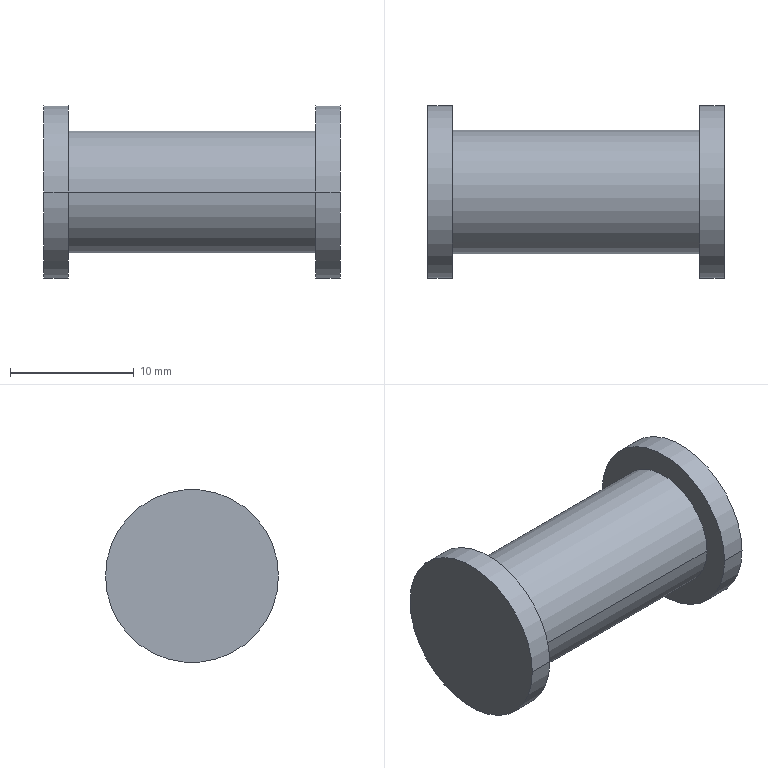Part | SolidWorks | 1 solid | 10 faces | box 24 x 14 x 14 mm | volume 2187 mm3 | cylinder 6 | plane 4 | commonest cylinder face diameters 14 x4 10 x2
STEP:
#1=CARTESIAN_POINT('',(-10.,-7.,0.));
#2=VERTEX_POINT('',#1);
#3=CARTESIAN_POINT('',(-10.,7.,0.));
#4=VERTEX_POINT('',#3);
#5=CARTESIAN_POINT('',(-10.,0.,0.));
#6=DIRECTION('',(-1.,0.,0.));
#7=DIRECTION('',(0.,-1.,0.));
#8=AXIS2_PLACEMENT_3D('',#5,#6,#7);
#9=CIRCLE('',#8,7.);
#10=EDGE_CURVE('',#2,#4,#9,.T.);
#11=ORIENTED_EDGE('',*,*,#10,.T.);
#12=CARTESIAN_POINT('',(-12.,7.,0.));
#13=VERTEX_POINT('',#12);
#14=CARTESIAN_POINT('',(0.,7.,0.));
#15=DIRECTION('',(-1.,0.,0.));
#16=VECTOR('',#15,1000.);
#17=LINE('',#14,#16);
#18=EDGE_CURVE('',#4,#13,#17,.T.);
#19=ORIENTED_EDGE('',*,*,#18,.T.);
#20=CARTESIAN_POINT('',(-12.,-7.,0.));
#21=VERTEX_POINT('',#20);
#22=CARTESIAN_POINT('',(-12.,0.,0.));
#23=DIRECTION('',(-1.,0.,0.));
#24=DIRECTION('',(0.,-1.,0.));
#25=AXIS2_PLACEMENT_3D('',#22,#23,#24);
#26=CIRCLE('',#25,7.);
#27=EDGE_CURVE('',#21,#13,#26,.T.);
#28=ORIENTED_EDGE('',*,*,#27,.F.);
#29=CARTESIAN_POINT('',(0.,-7.,0.));
#30=DIRECTION('',(-1.,0.,0.));
#31=VECTOR('',#30,1000.);
#32=LINE('',#29,#31);
#33=EDGE_CURVE('',#2,#21,#32,.T.);
#34=ORIENTED_EDGE('',*,*,#33,.F.);
#35=EDGE_LOOP('',(#11,#19,#28,#34));
#36=FACE_OUTER_BOUND('',#35,.T.);
#37=CARTESIAN_POINT('',(0.,0.,0.));
#38=DIRECTION('',(-1.,0.,0.));
#39=DIRECTION('',(0.,-1.,0.));
#40=AXIS2_PLACEMENT_3D('',#37,#38,#39);
#41=CYLINDRICAL_SURFACE('',#40,7.);
#42=ADVANCED_FACE('',(#36),#41,.T.);
#43=CARTESIAN_POINT('',(12.,-7.,0.));
#44=VERTEX_POINT('',#43);
#45=CARTESIAN_POINT('',(12.,7.,0.));
#46=VERTEX_POINT('',#45);
#47=CARTESIAN_POINT('',(12.,0.,0.));
#48=DIRECTION('',(-1.,0.,0.));
#49=DIRECTION('',(0.,-1.,0.));
#50=AXIS2_PLACEMENT_3D('',#47,#48,#49);
#51=CIRCLE('',#50,7.);
#52=EDGE_CURVE('',#44,#46,#51,.T.);
#53=ORIENTED_EDGE('',*,*,#52,.T.);
#54=CARTESIAN_POINT('',(10.,7.,0.));
#55=VERTEX_POINT('',#54);
#56=CARTESIAN_POINT('',(0.,7.,0.));
#57=DIRECTION('',(-1.,0.,0.));
#58=VECTOR('',#57,1000.);
#59=LINE('',#56,#58);
#60=EDGE_CURVE('',#46,#55,#59,.T.);
#61=ORIENTED_EDGE('',*,*,#60,.T.);
#62=CARTESIAN_POINT('',(10.,-7.,0.));
#63=VERTEX_POINT('',#62);
#64=CARTESIAN_POINT('',(10.,0.,0.));
#65=DIRECTION('',(-1.,0.,0.));
#66=DIRECTION('',(0.,-1.,0.));
#67=AXIS2_PLACEMENT_3D('',#64,#65,#66);
#68=CIRCLE('',#67,7.);
#69=EDGE_CURVE('',#63,#55,#68,.T.);
#70=ORIENTED_EDGE('',*,*,#69,.F.);
#71=CARTESIAN_POINT('',(0.,-7.,0.));
#72=DIRECTION('',(-1.,0.,0.));
#73=VECTOR('',#72,1000.);
#74=LINE('',#71,#73);
#75=EDGE_CURVE('',#44,#63,#74,.T.);
#76=ORIENTED_EDGE('',*,*,#75,.F.);
#77=EDGE_LOOP('',(#53,#61,#70,#76));
#78=FACE_OUTER_BOUND('',#77,.T.);
#79=CARTESIAN_POINT('',(0.,0.,0.));
#80=DIRECTION('',(-1.,0.,0.));
#81=DIRECTION('',(0.,-1.,0.));
#82=AXIS2_PLACEMENT_3D('',#79,#80,#81);
#83=CYLINDRICAL_SURFACE('',#82,7.);
#84=ADVANCED_FACE('',(#78),#83,.T.);
#85=CARTESIAN_POINT('',(10.,-5.,0.));
#86=VERTEX_POINT('',#85);
#87=CARTESIAN_POINT('',(10.,5.,0.));
#88=VERTEX_POINT('',#87);
#89=CARTESIAN_POINT('',(10.,0.,0.));
#90=DIRECTION('',(-1.,0.,0.));
#91=DIRECTION('',(0.,-1.,0.));
#92=AXIS2_PLACEMENT_3D('',#89,#90,#91);
#93=CIRCLE('',#92,5.);
#94=EDGE_CURVE('',#86,#88,#93,.T.);
#95=ORIENTED_EDGE('',*,*,#94,.T.);
#96=CARTESIAN_POINT('',(-10.,5.,0.));
#97=VERTEX_POINT('',#96);
#98=CARTESIAN_POINT('',(0.,5.,0.));
#99=DIRECTION('',(-1.,0.,0.));
#100=VECTOR('',#99,1000.);
#101=LINE('',#98,#100);
#102=EDGE_CURVE('',#88,#97,#101,.T.);
#103=ORIENTED_EDGE('',*,*,#102,.T.);
#104=CARTESIAN_POINT('',(-10.,-5.,0.));
#105=VERTEX_POINT('',#104);
#106=CARTESIAN_POINT('',(-10.,0.,0.));
#107=DIRECTION('',(-1.,0.,0.));
#108=DIRECTION('',(0.,-1.,0.));
#109=AXIS2_PLACEMENT_3D('',#106,#107,#108);
#110=CIRCLE('',#109,5.);
#111=EDGE_CURVE('',#105,#97,#110,.T.);
#112=ORIENTED_EDGE('',*,*,#111,.F.);
#113=CARTESIAN_POINT('',(0.,-5.,0.));
#114=DIRECTION('',(-1.,0.,0.));
#115=VECTOR('',#114,1000.);
#116=LINE('',#113,#115);
#117=EDGE_CURVE('',#86,#105,#116,.T.);
#118=ORIENTED_EDGE('',*,*,#117,.F.);
#119=EDGE_LOOP('',(#95,#103,#112,#118));
#120=FACE_OUTER_BOUND('',#119,.T.);
#121=CARTESIAN_POINT('',(0.,0.,0.));
#122=DIRECTION('',(-1.,0.,0.));
#123=DIRECTION('',(0.,-1.,0.));
#124=AXIS2_PLACEMENT_3D('',#121,#122,#123);
#125=CYLINDRICAL_SURFACE('',#124,5.);
#126=ADVANCED_FACE('',(#120),#125,.T.);
#127=ORIENTED_EDGE('',*,*,#10,.F.);
#128=CARTESIAN_POINT('',(-10.,0.,0.));
#129=DIRECTION('',(-1.,0.,0.));
#130=DIRECTION('',(0.,-1.,0.));
#131=AXIS2_PLACEMENT_3D('',#128,#129,#130);
#132=CIRCLE('',#131,7.);
#133=EDGE_CURVE('',#4,#2,#132,.T.);
#134=ORIENTED_EDGE('',*,*,#133,.F.);
#135=EDGE_LOOP('',(#127,#134));
#136=FACE_OUTER_BOUND('',#135,.T.);
#137=ORIENTED_EDGE('',*,*,#111,.T.);
#138=CARTESIAN_POINT('',(-10.,0.,0.));
#139=DIRECTION('',(-1.,0.,0.));
#140=DIRECTION('',(0.,-1.,0.));
#141=AXIS2_PLACEMENT_3D('',#138,#139,#140);
#142=CIRCLE('',#141,5.);
#143=EDGE_CURVE('',#97,#105,#142,.T.);
#144=ORIENTED_EDGE('',*,*,#143,.T.);
#145=EDGE_LOOP('',(#137,#144));
#146=FACE_BOUND('',#145,.T.);
#147=CARTESIAN_POINT('',(-10.,5.,0.));
#148=DIRECTION('',(-1.,0.,0.));
#149=DIRECTION('',(0.,-1.,0.));
#150=AXIS2_PLACEMENT_3D('',#147,#148,#149);
#151=PLANE('',#150);
#152=ADVANCED_FACE('',(#136,#146),#151,.F.);
#153=ORIENTED_EDGE('',*,*,#102,.F.);
#154=CARTESIAN_POINT('',(10.,0.,0.));
#155=DIRECTION('',(-1.,0.,0.));
#156=DIRECTION('',(0.,-1.,0.));
#157=AXIS2_PLACEMENT_3D('',#154,#155,#156);
#158=CIRCLE('',#157,5.);
#159=EDGE_CURVE('',#88,#86,#158,.T.);
#160=ORIENTED_EDGE('',*,*,#159,.T.);
#161=ORIENTED_EDGE('',*,*,#117,.T.);
#162=ORIENTED_EDGE('',*,*,#143,.F.);
#163=EDGE_LOOP('',(#153,#160,#161,#162));
#164=FACE_OUTER_BOUND('',#163,.T.);
#165=CARTESIAN_POINT('',(0.,0.,0.));
#166=DIRECTION('',(-1.,0.,0.));
#167=DIRECTION('',(0.,-1.,0.));
#168=AXIS2_PLACEMENT_3D('',#165,#166,#167);
#169=CYLINDRICAL_SURFACE('',#168,5.);
#170=ADVANCED_FACE('',(#164),#169,.T.);
#171=ORIENTED_EDGE('',*,*,#94,.F.);
#172=ORIENTED_EDGE('',*,*,#159,.F.);
#173=EDGE_LOOP('',(#171,#172));
#174=FACE_BOUND('',#173,.T.);
#175=ORIENTED_EDGE('',*,*,#69,.T.);
#176=CARTESIAN_POINT('',(10.,0.,0.));
#177=DIRECTION('',(-1.,0.,0.));
#178=DIRECTION('',(0.,-1.,0.));
#179=AXIS2_PLACEMENT_3D('',#176,#177,#178);
#180=CIRCLE('',#179,7.);
#181=EDGE_CURVE('',#55,#63,#180,.T.);
#182=ORIENTED_EDGE('',*,*,#181,.T.);
#183=EDGE_LOOP('',(#175,#182));
#184=FACE_OUTER_BOUND('',#183,.T.);
#185=CARTESIAN_POINT('',(10.,5.,0.));
#186=DIRECTION('',(1.,0.,0.));
#187=DIRECTION('',(0.,1.,0.));
#188=AXIS2_PLACEMENT_3D('',#185,#186,#187);
#189=PLANE('',#188);
#190=ADVANCED_FACE('',(#174,#184),#189,.F.);
#191=ORIENTED_EDGE('',*,*,#60,.F.);
#192=CARTESIAN_POINT('',(12.,0.,0.));
#193=DIRECTION('',(-1.,0.,0.));
#194=DIRECTION('',(0.,-1.,0.));
#195=AXIS2_PLACEMENT_3D('',#192,#193,#194);
#196=CIRCLE('',#195,7.);
#197=EDGE_CURVE('',#46,#44,#196,.T.);
#198=ORIENTED_EDGE('',*,*,#197,.T.);
#199=ORIENTED_EDGE('',*,*,#75,.T.);
#200=ORIENTED_EDGE('',*,*,#181,.F.);
#201=EDGE_LOOP('',(#191,#198,#199,#200));
#202=FACE_OUTER_BOUND('',#201,.T.);
#203=CARTESIAN_POINT('',(0.,0.,0.));
#204=DIRECTION('',(-1.,0.,0.));
#205=DIRECTION('',(0.,-1.,0.));
#206=AXIS2_PLACEMENT_3D('',#203,#204,#205);
#207=CYLINDRICAL_SURFACE('',#206,7.);
#208=ADVANCED_FACE('',(#202),#207,.T.);
#209=ORIENTED_EDGE('',*,*,#52,.F.);
#210=ORIENTED_EDGE('',*,*,#197,.F.);
#211=EDGE_LOOP('',(#209,#210));
#212=FACE_OUTER_BOUND('',#211,.T.);
#213=CARTESIAN_POINT('',(12.,7.,0.));
#214=DIRECTION('',(-1.,0.,0.));
#215=DIRECTION('',(0.,-1.,0.));
#216=AXIS2_PLACEMENT_3D('',#213,#214,#215);
#217=PLANE('',#216);
#218=ADVANCED_FACE('',(#212),#217,.F.);
#219=ORIENTED_EDGE('',*,*,#27,.T.);
#220=CARTESIAN_POINT('',(-12.,0.,0.));
#221=DIRECTION('',(-1.,0.,0.));
#222=DIRECTION('',(0.,-1.,0.));
#223=AXIS2_PLACEMENT_3D('',#220,#221,#222);
#224=CIRCLE('',#223,7.);
#225=EDGE_CURVE('',#13,#21,#224,.T.);
#226=ORIENTED_EDGE('',*,*,#225,.T.);
#227=EDGE_LOOP('',(#219,#226));
#228=FACE_OUTER_BOUND('',#227,.T.);
#229=CARTESIAN_POINT('',(-12.,7.,0.));
#230=DIRECTION('',(1.,0.,0.));
#231=DIRECTION('',(0.,1.,0.));
#232=AXIS2_PLACEMENT_3D('',#229,#230,#231);
#233=PLANE('',#232);
#234=ADVANCED_FACE('',(#228),#233,.F.);
#235=ORIENTED_EDGE('',*,*,#18,.F.);
#236=ORIENTED_EDGE('',*,*,#133,.T.);
#237=ORIENTED_EDGE('',*,*,#33,.T.);
#238=ORIENTED_EDGE('',*,*,#225,.F.);
#239=EDGE_LOOP('',(#235,#236,#237,#238));
#240=FACE_OUTER_BOUND('',#239,.T.);
#241=CARTESIAN_POINT('',(0.,0.,0.));
#242=DIRECTION('',(-1.,0.,0.));
#243=DIRECTION('',(0.,-1.,0.));
#244=AXIS2_PLACEMENT_3D('',#241,#242,#243);
#245=CYLINDRICAL_SURFACE('',#244,7.);
#246=ADVANCED_FACE('',(#240),#245,.T.);
#247=CLOSED_SHELL('',(#42,#84,#126,#152,#170,#190,#208,#218,#234,#246));
#248=MANIFOLD_SOLID_BREP('',#247);
#249=CARTESIAN_POINT('',(0.,0.,0.));
#250=DIRECTION('',(0.,0.,1.));
#251=DIRECTION('',(1.,0.,0.));
#252=AXIS2_PLACEMENT_3D('',#249,#250,#251);
#253=(LENGTH_UNIT()NAMED_UNIT(*)SI_UNIT(.MILLI.,.METRE.));
#254=UNCERTAINTY_MEASURE_WITH_UNIT(LENGTH_MEASURE(0.00001),#253,'','');
#255=(NAMED_UNIT(*)PLANE_ANGLE_UNIT()SI_UNIT($,.RADIAN.));
#256=(NAMED_UNIT(*)SI_UNIT($,.STERADIAN.)SOLID_ANGLE_UNIT());
#257=(GEOMETRIC_REPRESENTATION_CONTEXT(3)GLOBAL_UNCERTAINTY_ASSIGNED_CONTEXT((#254))GLOBAL_UNIT_ASSIGNED_CONTEXT((#253,#255,#256))REPRESENTATION_CONTEXT('',''));
#258=ADVANCED_BREP_SHAPE_REPRESENTATION('',(#248,#252),#257);